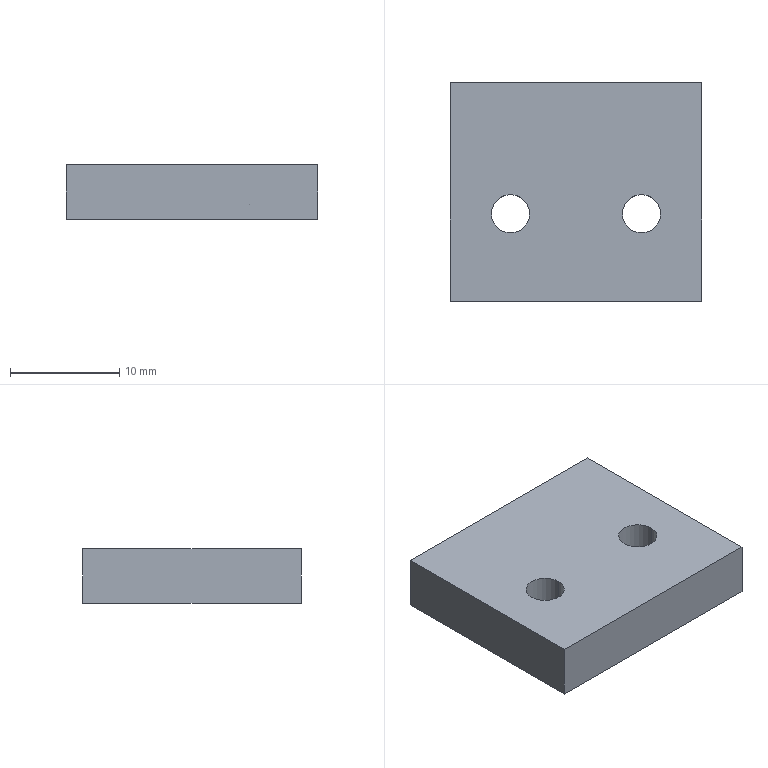Part | STEP file | Shift cylinder pad | 1 solid | 10 faces | box 23 x 20 x 5 mm | volume 2204 mm3 | plane 6 | cylinder 4 | commonest cylinder face diameters 3.5 x4
STEP:
#1=CARTESIAN_POINT('',(0.,0.,0.));
#2=DIRECTION('',(0.,0.,1.));
#3=DIRECTION('',(1.,0.,0.));
#4=AXIS2_PLACEMENT_3D('',#1,#2,#3);
#5=CARTESIAN_POINT('',(7.25,8.,0.));
#6=VERTEX_POINT('',#5);
#7=CARTESIAN_POINT('',(7.25,8.,5.));
#8=VERTEX_POINT('',#7);
#9=CARTESIAN_POINT('',(7.25,8.,0.));
#10=DIRECTION('',(0.,0.,1.));
#11=VECTOR('',#10,1.);
#12=LINE('',#9,#11);
#13=CARTESIAN_POINT('',(5.5,8.,0.));
#14=DIRECTION('',(0.,0.,1.));
#15=DIRECTION('',(1.,0.,0.));
#16=AXIS2_PLACEMENT_3D('',#13,#14,#15);
#17=CYLINDRICAL_SURFACE('',#16,1.75);
#18=CARTESIAN_POINT('',(6.283,0.));
#19=DIRECTION('',(0.,1.));
#20=VECTOR('',#19,1.);
#21=LINE('',#18,#20);
#22=(GEOMETRIC_REPRESENTATION_CONTEXT(2)PARAMETRIC_REPRESENTATION_CONTEXT()REPRESENTATION_CONTEXT('',''));
#23=DEFINITIONAL_REPRESENTATION('',(#21),#22);
#24=PCURVE('',#17,#23);
#25=CARTESIAN_POINT('',(5.5,8.,0.));
#26=DIRECTION('',(0.,0.,1.));
#27=DIRECTION('',(1.,0.,0.));
#28=AXIS2_PLACEMENT_3D('',#25,#26,#27);
#29=CYLINDRICAL_SURFACE('',#28,1.75);
#30=CARTESIAN_POINT('',(0.,0.));
#31=DIRECTION('',(0.,1.));
#32=VECTOR('',#31,1.);
#33=LINE('',#30,#32);
#34=(GEOMETRIC_REPRESENTATION_CONTEXT(2)PARAMETRIC_REPRESENTATION_CONTEXT()REPRESENTATION_CONTEXT('',''));
#35=DEFINITIONAL_REPRESENTATION('',(#33),#34);
#36=PCURVE('',#29,#35);
#37=SURFACE_CURVE('',#12,(#24,#36),.PCURVE_S1.);
#38=EDGE_CURVE('',#6,#8,#37,.T.);
#39=ORIENTED_EDGE('',*,*,#38,.T.);
#40=CARTESIAN_POINT('',(3.75,8.,5.));
#41=VERTEX_POINT('',#40);
#42=CARTESIAN_POINT('',(5.5,8.,5.));
#43=DIRECTION('',(0.,0.,1.));
#44=DIRECTION('',(1.,0.,0.));
#45=AXIS2_PLACEMENT_3D('',#42,#43,#44);
#46=CIRCLE('',#45,1.75);
#47=CARTESIAN_POINT('',(0.,5.));
#48=DIRECTION('',(1.,0.));
#49=VECTOR('',#48,1.);
#50=LINE('',#47,#49);
#51=(GEOMETRIC_REPRESENTATION_CONTEXT(2)PARAMETRIC_REPRESENTATION_CONTEXT()REPRESENTATION_CONTEXT('',''));
#52=DEFINITIONAL_REPRESENTATION('',(#50),#51);
#53=PCURVE('',#17,#52);
#54=CARTESIAN_POINT('',(0.,20.,5.));
#55=DIRECTION('',(0.,0.,-1.));
#56=DIRECTION('',(-1.,0.,0.));
#57=AXIS2_PLACEMENT_3D('',#54,#55,#56);
#58=PLANE('',#57);
#59=CARTESIAN_POINT('',(-7.25,-12.));
#60=CARTESIAN_POINT('',(-7.25,-8.969));
#61=CARTESIAN_POINT('',(-4.625,-10.484));
#62=CARTESIAN_POINT('',(-2.,-12.));
#63=CARTESIAN_POINT('',(-4.625,-13.516));
#64=CARTESIAN_POINT('',(-7.25,-15.031));
#65=CARTESIAN_POINT('',(-7.25,-12.));
#66=(BOUNDED_CURVE()B_SPLINE_CURVE(2,(#59,#60,#61,#62,#63,#64,#65),.UNSPECIFIED.,.T.,.F.)B_SPLINE_CURVE_WITH_KNOTS((1,2,2,2,2,1),(-2.094,0.,2.094,4.189,6.283,8.378),.UNSPECIFIED.)CURVE()GEOMETRIC_REPRESENTATION_ITEM()RATIONAL_B_SPLINE_CURVE((1.,0.5,1.,0.5,1.,0.5,1.))REPRESENTATION_ITEM(''));
#67=(GEOMETRIC_REPRESENTATION_CONTEXT(2)PARAMETRIC_REPRESENTATION_CONTEXT()REPRESENTATION_CONTEXT('',''));
#68=DEFINITIONAL_REPRESENTATION('',(#66),#67);
#69=PCURVE('',#58,#68);
#70=SURFACE_CURVE('',#46,(#53,#69),.PCURVE_S1.);
#71=EDGE_CURVE('',#41,#8,#70,.T.);
#72=ORIENTED_EDGE('',*,*,#71,.F.);
#73=CARTESIAN_POINT('',(3.75,8.,0.));
#74=VERTEX_POINT('',#73);
#75=CARTESIAN_POINT('',(3.75,8.,0.));
#76=DIRECTION('',(0.,0.,1.));
#77=VECTOR('',#76,1.);
#78=LINE('',#75,#77);
#79=CARTESIAN_POINT('',(3.142,0.));
#80=DIRECTION('',(0.,1.));
#81=VECTOR('',#80,1.);
#82=LINE('',#79,#81);
#83=(GEOMETRIC_REPRESENTATION_CONTEXT(2)PARAMETRIC_REPRESENTATION_CONTEXT()REPRESENTATION_CONTEXT('',''));
#84=DEFINITIONAL_REPRESENTATION('',(#82),#83);
#85=PCURVE('',#17,#84);
#86=CARTESIAN_POINT('',(3.142,0.));
#87=DIRECTION('',(0.,1.));
#88=VECTOR('',#87,1.);
#89=LINE('',#86,#88);
#90=(GEOMETRIC_REPRESENTATION_CONTEXT(2)PARAMETRIC_REPRESENTATION_CONTEXT()REPRESENTATION_CONTEXT('',''));
#91=DEFINITIONAL_REPRESENTATION('',(#89),#90);
#92=PCURVE('',#29,#91);
#93=SURFACE_CURVE('',#78,(#85,#92),.PCURVE_S1.);
#94=EDGE_CURVE('',#74,#41,#93,.T.);
#95=ORIENTED_EDGE('',*,*,#94,.F.);
#96=CARTESIAN_POINT('',(5.5,8.,0.));
#97=DIRECTION('',(0.,0.,1.));
#98=DIRECTION('',(1.,0.,0.));
#99=AXIS2_PLACEMENT_3D('',#96,#97,#98);
#100=CIRCLE('',#99,1.75);
#101=CARTESIAN_POINT('',(0.,0.));
#102=DIRECTION('',(1.,0.));
#103=VECTOR('',#102,1.);
#104=LINE('',#101,#103);
#105=(GEOMETRIC_REPRESENTATION_CONTEXT(2)PARAMETRIC_REPRESENTATION_CONTEXT()REPRESENTATION_CONTEXT('',''));
#106=DEFINITIONAL_REPRESENTATION('',(#104),#105);
#107=PCURVE('',#17,#106);
#108=CARTESIAN_POINT('',(0.,20.,0.));
#109=DIRECTION('',(0.,0.,-1.));
#110=DIRECTION('',(-1.,0.,0.));
#111=AXIS2_PLACEMENT_3D('',#108,#109,#110);
#112=PLANE('',#111);
#113=CARTESIAN_POINT('',(-7.25,-12.));
#114=CARTESIAN_POINT('',(-7.25,-8.969));
#115=CARTESIAN_POINT('',(-4.625,-10.484));
#116=CARTESIAN_POINT('',(-2.,-12.));
#117=CARTESIAN_POINT('',(-4.625,-13.516));
#118=CARTESIAN_POINT('',(-7.25,-15.031));
#119=CARTESIAN_POINT('',(-7.25,-12.));
#120=(BOUNDED_CURVE()B_SPLINE_CURVE(2,(#113,#114,#115,#116,#117,#118,#119),.UNSPECIFIED.,.T.,.F.)B_SPLINE_CURVE_WITH_KNOTS((1,2,2,2,2,1),(-2.094,0.,2.094,4.189,6.283,8.378),.UNSPECIFIED.)CURVE()GEOMETRIC_REPRESENTATION_ITEM()RATIONAL_B_SPLINE_CURVE((1.,0.5,1.,0.5,1.,0.5,1.))REPRESENTATION_ITEM(''));
#121=(GEOMETRIC_REPRESENTATION_CONTEXT(2)PARAMETRIC_REPRESENTATION_CONTEXT()REPRESENTATION_CONTEXT('',''));
#122=DEFINITIONAL_REPRESENTATION('',(#120),#121);
#123=PCURVE('',#112,#122);
#124=SURFACE_CURVE('',#100,(#107,#123),.PCURVE_S1.);
#125=EDGE_CURVE('',#74,#6,#124,.T.);
#126=ORIENTED_EDGE('',*,*,#125,.T.);
#127=EDGE_LOOP('',(#39,#72,#95,#126));
#128=FACE_BOUND('',#127,.F.);
#129=ADVANCED_FACE('',(#128),#17,.F.);
#130=CARTESIAN_POINT('',(19.25,8.,0.));
#131=VERTEX_POINT('',#130);
#132=CARTESIAN_POINT('',(19.25,8.,5.));
#133=VERTEX_POINT('',#132);
#134=CARTESIAN_POINT('',(19.25,8.,0.));
#135=DIRECTION('',(0.,0.,1.));
#136=VECTOR('',#135,1.);
#137=LINE('',#134,#136);
#138=CARTESIAN_POINT('',(17.5,8.,0.));
#139=DIRECTION('',(0.,0.,1.));
#140=DIRECTION('',(1.,0.,0.));
#141=AXIS2_PLACEMENT_3D('',#138,#139,#140);
#142=CYLINDRICAL_SURFACE('',#141,1.75);
#143=CARTESIAN_POINT('',(6.283,0.));
#144=DIRECTION('',(0.,1.));
#145=VECTOR('',#144,1.);
#146=LINE('',#143,#145);
#147=(GEOMETRIC_REPRESENTATION_CONTEXT(2)PARAMETRIC_REPRESENTATION_CONTEXT()REPRESENTATION_CONTEXT('',''));
#148=DEFINITIONAL_REPRESENTATION('',(#146),#147);
#149=PCURVE('',#142,#148);
#150=CARTESIAN_POINT('',(17.5,8.,0.));
#151=DIRECTION('',(0.,0.,1.));
#152=DIRECTION('',(1.,0.,0.));
#153=AXIS2_PLACEMENT_3D('',#150,#151,#152);
#154=CYLINDRICAL_SURFACE('',#153,1.75);
#155=CARTESIAN_POINT('',(0.,0.));
#156=DIRECTION('',(0.,1.));
#157=VECTOR('',#156,1.);
#158=LINE('',#155,#157);
#159=(GEOMETRIC_REPRESENTATION_CONTEXT(2)PARAMETRIC_REPRESENTATION_CONTEXT()REPRESENTATION_CONTEXT('',''));
#160=DEFINITIONAL_REPRESENTATION('',(#158),#159);
#161=PCURVE('',#154,#160);
#162=SURFACE_CURVE('',#137,(#149,#161),.PCURVE_S1.);
#163=EDGE_CURVE('',#131,#133,#162,.T.);
#164=ORIENTED_EDGE('',*,*,#163,.T.);
#165=CARTESIAN_POINT('',(15.75,8.,5.));
#166=VERTEX_POINT('',#165);
#167=CARTESIAN_POINT('',(17.5,8.,5.));
#168=DIRECTION('',(0.,0.,1.));
#169=DIRECTION('',(1.,0.,0.));
#170=AXIS2_PLACEMENT_3D('',#167,#168,#169);
#171=CIRCLE('',#170,1.75);
#172=CARTESIAN_POINT('',(0.,5.));
#173=DIRECTION('',(1.,0.));
#174=VECTOR('',#173,1.);
#175=LINE('',#172,#174);
#176=(GEOMETRIC_REPRESENTATION_CONTEXT(2)PARAMETRIC_REPRESENTATION_CONTEXT()REPRESENTATION_CONTEXT('',''));
#177=DEFINITIONAL_REPRESENTATION('',(#175),#176);
#178=PCURVE('',#142,#177);
#179=CARTESIAN_POINT('',(-19.25,-12.));
#180=CARTESIAN_POINT('',(-19.25,-8.969));
#181=CARTESIAN_POINT('',(-16.625,-10.484));
#182=CARTESIAN_POINT('',(-14.,-12.));
#183=CARTESIAN_POINT('',(-16.625,-13.516));
#184=CARTESIAN_POINT('',(-19.25,-15.031));
#185=CARTESIAN_POINT('',(-19.25,-12.));
#186=(BOUNDED_CURVE()B_SPLINE_CURVE(2,(#179,#180,#181,#182,#183,#184,#185),.UNSPECIFIED.,.T.,.F.)B_SPLINE_CURVE_WITH_KNOTS((1,2,2,2,2,1),(-2.094,0.,2.094,4.189,6.283,8.378),.UNSPECIFIED.)CURVE()GEOMETRIC_REPRESENTATION_ITEM()RATIONAL_B_SPLINE_CURVE((1.,0.5,1.,0.5,1.,0.5,1.))REPRESENTATION_ITEM(''));
#187=(GEOMETRIC_REPRESENTATION_CONTEXT(2)PARAMETRIC_REPRESENTATION_CONTEXT()REPRESENTATION_CONTEXT('',''));
#188=DEFINITIONAL_REPRESENTATION('',(#186),#187);
#189=PCURVE('',#58,#188);
#190=SURFACE_CURVE('',#171,(#178,#189),.PCURVE_S1.);
#191=EDGE_CURVE('',#166,#133,#190,.T.);
#192=ORIENTED_EDGE('',*,*,#191,.F.);
#193=CARTESIAN_POINT('',(15.75,8.,0.));
#194=VERTEX_POINT('',#193);
#195=CARTESIAN_POINT('',(15.75,8.,0.));
#196=DIRECTION('',(0.,0.,1.));
#197=VECTOR('',#196,1.);
#198=LINE('',#195,#197);
#199=CARTESIAN_POINT('',(3.142,0.));
#200=DIRECTION('',(0.,1.));
#201=VECTOR('',#200,1.);
#202=LINE('',#199,#201);
#203=(GEOMETRIC_REPRESENTATION_CONTEXT(2)PARAMETRIC_REPRESENTATION_CONTEXT()REPRESENTATION_CONTEXT('',''));
#204=DEFINITIONAL_REPRESENTATION('',(#202),#203);
#205=PCURVE('',#142,#204);
#206=CARTESIAN_POINT('',(3.142,0.));
#207=DIRECTION('',(0.,1.));
#208=VECTOR('',#207,1.);
#209=LINE('',#206,#208);
#210=(GEOMETRIC_REPRESENTATION_CONTEXT(2)PARAMETRIC_REPRESENTATION_CONTEXT()REPRESENTATION_CONTEXT('',''));
#211=DEFINITIONAL_REPRESENTATION('',(#209),#210);
#212=PCURVE('',#154,#211);
#213=SURFACE_CURVE('',#198,(#205,#212),.PCURVE_S1.);
#214=EDGE_CURVE('',#194,#166,#213,.T.);
#215=ORIENTED_EDGE('',*,*,#214,.F.);
#216=CARTESIAN_POINT('',(17.5,8.,0.));
#217=DIRECTION('',(0.,0.,1.));
#218=DIRECTION('',(1.,0.,0.));
#219=AXIS2_PLACEMENT_3D('',#216,#217,#218);
#220=CIRCLE('',#219,1.75);
#221=CARTESIAN_POINT('',(0.,0.));
#222=DIRECTION('',(1.,0.));
#223=VECTOR('',#222,1.);
#224=LINE('',#221,#223);
#225=(GEOMETRIC_REPRESENTATION_CONTEXT(2)PARAMETRIC_REPRESENTATION_CONTEXT()REPRESENTATION_CONTEXT('',''));
#226=DEFINITIONAL_REPRESENTATION('',(#224),#225);
#227=PCURVE('',#142,#226);
#228=CARTESIAN_POINT('',(-19.25,-12.));
#229=CARTESIAN_POINT('',(-19.25,-8.969));
#230=CARTESIAN_POINT('',(-16.625,-10.484));
#231=CARTESIAN_POINT('',(-14.,-12.));
#232=CARTESIAN_POINT('',(-16.625,-13.516));
#233=CARTESIAN_POINT('',(-19.25,-15.031));
#234=CARTESIAN_POINT('',(-19.25,-12.));
#235=(BOUNDED_CURVE()B_SPLINE_CURVE(2,(#228,#229,#230,#231,#232,#233,#234),.UNSPECIFIED.,.T.,.F.)B_SPLINE_CURVE_WITH_KNOTS((1,2,2,2,2,1),(-2.094,0.,2.094,4.189,6.283,8.378),.UNSPECIFIED.)CURVE()GEOMETRIC_REPRESENTATION_ITEM()RATIONAL_B_SPLINE_CURVE((1.,0.5,1.,0.5,1.,0.5,1.))REPRESENTATION_ITEM(''));
#236=(GEOMETRIC_REPRESENTATION_CONTEXT(2)PARAMETRIC_REPRESENTATION_CONTEXT()REPRESENTATION_CONTEXT('',''));
#237=DEFINITIONAL_REPRESENTATION('',(#235),#236);
#238=PCURVE('',#112,#237);
#239=SURFACE_CURVE('',#220,(#227,#238),.PCURVE_S1.);
#240=EDGE_CURVE('',#194,#131,#239,.T.);
#241=ORIENTED_EDGE('',*,*,#240,.T.);
#242=EDGE_LOOP('',(#164,#192,#215,#241));
#243=FACE_BOUND('',#242,.F.);
#244=ADVANCED_FACE('',(#243),#142,.F.);
#245=CARTESIAN_POINT('',(0.,20.,0.));
#246=VERTEX_POINT('',#245);
#247=CARTESIAN_POINT('',(0.,0.,0.));
#248=VERTEX_POINT('',#247);
#249=CARTESIAN_POINT('',(0.,0.,0.));
#250=DIRECTION('',(0.,-1.,0.));
#251=VECTOR('',#250,1.);
#252=LINE('',#249,#251);
#253=CARTESIAN_POINT('',(0.,0.,5.));
#254=DIRECTION('',(1.,0.,0.));
#255=DIRECTION('',(0.,0.,-1.));
#256=AXIS2_PLACEMENT_3D('',#253,#254,#255);
#257=PLANE('',#256);
#258=CARTESIAN_POINT('',(5.,0.));
#259=DIRECTION('',(0.,-1.));
#260=VECTOR('',#259,1.);
#261=LINE('',#258,#260);
#262=(GEOMETRIC_REPRESENTATION_CONTEXT(2)PARAMETRIC_REPRESENTATION_CONTEXT()REPRESENTATION_CONTEXT('',''));
#263=DEFINITIONAL_REPRESENTATION('',(#261),#262);
#264=PCURVE('',#257,#263);
#265=CARTESIAN_POINT('',(0.,-20.));
#266=DIRECTION('',(0.,-1.));
#267=VECTOR('',#266,1.);
#268=LINE('',#265,#267);
#269=(GEOMETRIC_REPRESENTATION_CONTEXT(2)PARAMETRIC_REPRESENTATION_CONTEXT()REPRESENTATION_CONTEXT('',''));
#270=DEFINITIONAL_REPRESENTATION('',(#268),#269);
#271=PCURVE('',#112,#270);
#272=SURFACE_CURVE('',#252,(#264,#271),.PCURVE_S1.);
#273=EDGE_CURVE('',#246,#248,#272,.T.);
#274=ORIENTED_EDGE('',*,*,#273,.T.);
#275=CARTESIAN_POINT('',(0.,0.,5.));
#276=VERTEX_POINT('',#275);
#277=CARTESIAN_POINT('',(0.,0.,5.));
#278=DIRECTION('',(0.,0.,-1.));
#279=VECTOR('',#278,1.);
#280=LINE('',#277,#279);
#281=CARTESIAN_POINT('',(0.,0.));
#282=DIRECTION('',(1.,0.));
#283=VECTOR('',#282,1.);
#284=LINE('',#281,#283);
#285=(GEOMETRIC_REPRESENTATION_CONTEXT(2)PARAMETRIC_REPRESENTATION_CONTEXT()REPRESENTATION_CONTEXT('',''));
#286=DEFINITIONAL_REPRESENTATION('',(#284),#285);
#287=PCURVE('',#257,#286);
#288=CARTESIAN_POINT('',(0.,0.,5.));
#289=DIRECTION('',(0.,1.,0.));
#290=DIRECTION('',(0.,0.,1.));
#291=AXIS2_PLACEMENT_3D('',#288,#289,#290);
#292=PLANE('',#291);
#293=CARTESIAN_POINT('',(0.,0.));
#294=DIRECTION('',(-1.,0.));
#295=VECTOR('',#294,1.);
#296=LINE('',#293,#295);
#297=(GEOMETRIC_REPRESENTATION_CONTEXT(2)PARAMETRIC_REPRESENTATION_CONTEXT()REPRESENTATION_CONTEXT('',''));
#298=DEFINITIONAL_REPRESENTATION('',(#296),#297);
#299=PCURVE('',#292,#298);
#300=SURFACE_CURVE('',#280,(#287,#299),.PCURVE_S1.);
#301=EDGE_CURVE('',#276,#248,#300,.T.);
#302=ORIENTED_EDGE('',*,*,#301,.F.);
#303=CARTESIAN_POINT('',(0.,20.,5.));
#304=VERTEX_POINT('',#303);
#305=CARTESIAN_POINT('',(0.,0.,5.));
#306=DIRECTION('',(0.,-1.,0.));
#307=VECTOR('',#306,1.);
#308=LINE('',#305,#307);
#309=CARTESIAN_POINT('',(0.,0.));
#310=DIRECTION('',(0.,-1.));
#311=VECTOR('',#310,1.);
#312=LINE('',#309,#311);
#313=(GEOMETRIC_REPRESENTATION_CONTEXT(2)PARAMETRIC_REPRESENTATION_CONTEXT()REPRESENTATION_CONTEXT('',''));
#314=DEFINITIONAL_REPRESENTATION('',(#312),#313);
#315=PCURVE('',#257,#314);
#316=CARTESIAN_POINT('',(0.,-20.));
#317=DIRECTION('',(0.,-1.));
#318=VECTOR('',#317,1.);
#319=LINE('',#316,#318);
#320=(GEOMETRIC_REPRESENTATION_CONTEXT(2)PARAMETRIC_REPRESENTATION_CONTEXT()REPRESENTATION_CONTEXT('',''));
#321=DEFINITIONAL_REPRESENTATION('',(#319),#320);
#322=PCURVE('',#58,#321);
#323=SURFACE_CURVE('',#308,(#315,#322),.PCURVE_S1.);
#324=EDGE_CURVE('',#304,#276,#323,.T.);
#325=ORIENTED_EDGE('',*,*,#324,.F.);
#326=CARTESIAN_POINT('',(0.,20.,5.));
#327=DIRECTION('',(0.,0.,-1.));
#328=VECTOR('',#327,1.);
#329=LINE('',#326,#328);
#330=CARTESIAN_POINT('',(0.,20.));
#331=DIRECTION('',(1.,0.));
#332=VECTOR('',#331,1.);
#333=LINE('',#330,#332);
#334=(GEOMETRIC_REPRESENTATION_CONTEXT(2)PARAMETRIC_REPRESENTATION_CONTEXT()REPRESENTATION_CONTEXT('',''));
#335=DEFINITIONAL_REPRESENTATION('',(#333),#334);
#336=PCURVE('',#257,#335);
#337=CARTESIAN_POINT('',(0.,20.,5.));
#338=DIRECTION('',(0.,-1.,0.));
#339=DIRECTION('',(0.,0.,-1.));
#340=AXIS2_PLACEMENT_3D('',#337,#338,#339);
#341=PLANE('',#340);
#342=CARTESIAN_POINT('',(0.,0.));
#343=DIRECTION('',(1.,0.));
#344=VECTOR('',#343,1.);
#345=LINE('',#342,#344);
#346=(GEOMETRIC_REPRESENTATION_CONTEXT(2)PARAMETRIC_REPRESENTATION_CONTEXT()REPRESENTATION_CONTEXT('',''));
#347=DEFINITIONAL_REPRESENTATION('',(#345),#346);
#348=PCURVE('',#341,#347);
#349=SURFACE_CURVE('',#329,(#336,#348),.PCURVE_S1.);
#350=EDGE_CURVE('',#304,#246,#349,.T.);
#351=ORIENTED_EDGE('',*,*,#350,.T.);
#352=EDGE_LOOP('',(#274,#302,#325,#351));
#353=FACE_BOUND('',#352,.T.);
#354=ADVANCED_FACE('',(#353),#257,.F.);
#355=CARTESIAN_POINT('',(23.,0.,0.));
#356=VERTEX_POINT('',#355);
#357=CARTESIAN_POINT('',(0.,0.,0.));
#358=DIRECTION('',(1.,0.,0.));
#359=VECTOR('',#358,1.);
#360=LINE('',#357,#359);
#361=CARTESIAN_POINT('',(-5.,0.));
#362=DIRECTION('',(0.,1.));
#363=VECTOR('',#362,1.);
#364=LINE('',#361,#363);
#365=(GEOMETRIC_REPRESENTATION_CONTEXT(2)PARAMETRIC_REPRESENTATION_CONTEXT()REPRESENTATION_CONTEXT('',''));
#366=DEFINITIONAL_REPRESENTATION('',(#364),#365);
#367=PCURVE('',#292,#366);
#368=CARTESIAN_POINT('',(0.,-20.));
#369=DIRECTION('',(-1.,0.));
#370=VECTOR('',#369,1.);
#371=LINE('',#368,#370);
#372=(GEOMETRIC_REPRESENTATION_CONTEXT(2)PARAMETRIC_REPRESENTATION_CONTEXT()REPRESENTATION_CONTEXT('',''));
#373=DEFINITIONAL_REPRESENTATION('',(#371),#372);
#374=PCURVE('',#112,#373);
#375=SURFACE_CURVE('',#360,(#367,#374),.PCURVE_S1.);
#376=EDGE_CURVE('',#248,#356,#375,.T.);
#377=ORIENTED_EDGE('',*,*,#376,.T.);
#378=CARTESIAN_POINT('',(23.,0.,5.));
#379=VERTEX_POINT('',#378);
#380=CARTESIAN_POINT('',(23.,0.,5.));
#381=DIRECTION('',(0.,0.,-1.));
#382=VECTOR('',#381,1.);
#383=LINE('',#380,#382);
#384=CARTESIAN_POINT('',(0.,23.));
#385=DIRECTION('',(-1.,0.));
#386=VECTOR('',#385,1.);
#387=LINE('',#384,#386);
#388=(GEOMETRIC_REPRESENTATION_CONTEXT(2)PARAMETRIC_REPRESENTATION_CONTEXT()REPRESENTATION_CONTEXT('',''));
#389=DEFINITIONAL_REPRESENTATION('',(#387),#388);
#390=PCURVE('',#292,#389);
#391=CARTESIAN_POINT('',(23.,0.,5.));
#392=DIRECTION('',(-1.,0.,0.));
#393=DIRECTION('',(0.,0.,1.));
#394=AXIS2_PLACEMENT_3D('',#391,#392,#393);
#395=PLANE('',#394);
#396=CARTESIAN_POINT('',(0.,0.));
#397=DIRECTION('',(-1.,0.));
#398=VECTOR('',#397,1.);
#399=LINE('',#396,#398);
#400=(GEOMETRIC_REPRESENTATION_CONTEXT(2)PARAMETRIC_REPRESENTATION_CONTEXT()REPRESENTATION_CONTEXT('',''));
#401=DEFINITIONAL_REPRESENTATION('',(#399),#400);
#402=PCURVE('',#395,#401);
#403=SURFACE_CURVE('',#383,(#390,#402),.PCURVE_S1.);
#404=EDGE_CURVE('',#379,#356,#403,.T.);
#405=ORIENTED_EDGE('',*,*,#404,.F.);
#406=CARTESIAN_POINT('',(0.,0.,5.));
#407=DIRECTION('',(1.,0.,0.));
#408=VECTOR('',#407,1.);
#409=LINE('',#406,#408);
#410=CARTESIAN_POINT('',(0.,0.));
#411=DIRECTION('',(0.,1.));
#412=VECTOR('',#411,1.);
#413=LINE('',#410,#412);
#414=(GEOMETRIC_REPRESENTATION_CONTEXT(2)PARAMETRIC_REPRESENTATION_CONTEXT()REPRESENTATION_CONTEXT('',''));
#415=DEFINITIONAL_REPRESENTATION('',(#413),#414);
#416=PCURVE('',#292,#415);
#417=CARTESIAN_POINT('',(0.,-20.));
#418=DIRECTION('',(-1.,0.));
#419=VECTOR('',#418,1.);
#420=LINE('',#417,#419);
#421=(GEOMETRIC_REPRESENTATION_CONTEXT(2)PARAMETRIC_REPRESENTATION_CONTEXT()REPRESENTATION_CONTEXT('',''));
#422=DEFINITIONAL_REPRESENTATION('',(#420),#421);
#423=PCURVE('',#58,#422);
#424=SURFACE_CURVE('',#409,(#416,#423),.PCURVE_S1.);
#425=EDGE_CURVE('',#276,#379,#424,.T.);
#426=ORIENTED_EDGE('',*,*,#425,.F.);
#427=ORIENTED_EDGE('',*,*,#301,.T.);
#428=EDGE_LOOP('',(#377,#405,#426,#427));
#429=FACE_BOUND('',#428,.T.);
#430=ADVANCED_FACE('',(#429),#292,.F.);
#431=CARTESIAN_POINT('',(23.,20.,0.));
#432=VERTEX_POINT('',#431);
#433=CARTESIAN_POINT('',(23.,0.,0.));
#434=DIRECTION('',(0.,1.,0.));
#435=VECTOR('',#434,1.);
#436=LINE('',#433,#435);
#437=CARTESIAN_POINT('',(-5.,0.));
#438=DIRECTION('',(0.,1.));
#439=VECTOR('',#438,1.);
#440=LINE('',#437,#439);
#441=(GEOMETRIC_REPRESENTATION_CONTEXT(2)PARAMETRIC_REPRESENTATION_CONTEXT()REPRESENTATION_CONTEXT('',''));
#442=DEFINITIONAL_REPRESENTATION('',(#440),#441);
#443=PCURVE('',#395,#442);
#444=CARTESIAN_POINT('',(-23.,-20.));
#445=DIRECTION('',(0.,1.));
#446=VECTOR('',#445,1.);
#447=LINE('',#444,#446);
#448=(GEOMETRIC_REPRESENTATION_CONTEXT(2)PARAMETRIC_REPRESENTATION_CONTEXT()REPRESENTATION_CONTEXT('',''));
#449=DEFINITIONAL_REPRESENTATION('',(#447),#448);
#450=PCURVE('',#112,#449);
#451=SURFACE_CURVE('',#436,(#443,#450),.PCURVE_S1.);
#452=EDGE_CURVE('',#356,#432,#451,.T.);
#453=ORIENTED_EDGE('',*,*,#452,.T.);
#454=CARTESIAN_POINT('',(23.,20.,5.));
#455=VERTEX_POINT('',#454);
#456=CARTESIAN_POINT('',(23.,20.,5.));
#457=DIRECTION('',(0.,0.,-1.));
#458=VECTOR('',#457,1.);
#459=LINE('',#456,#458);
#460=CARTESIAN_POINT('',(0.,20.));
#461=DIRECTION('',(-1.,0.));
#462=VECTOR('',#461,1.);
#463=LINE('',#460,#462);
#464=(GEOMETRIC_REPRESENTATION_CONTEXT(2)PARAMETRIC_REPRESENTATION_CONTEXT()REPRESENTATION_CONTEXT('',''));
#465=DEFINITIONAL_REPRESENTATION('',(#463),#464);
#466=PCURVE('',#395,#465);
#467=CARTESIAN_POINT('',(0.,23.));
#468=DIRECTION('',(1.,0.));
#469=VECTOR('',#468,1.);
#470=LINE('',#467,#469);
#471=(GEOMETRIC_REPRESENTATION_CONTEXT(2)PARAMETRIC_REPRESENTATION_CONTEXT()REPRESENTATION_CONTEXT('',''));
#472=DEFINITIONAL_REPRESENTATION('',(#470),#471);
#473=PCURVE('',#341,#472);
#474=SURFACE_CURVE('',#459,(#466,#473),.PCURVE_S1.);
#475=EDGE_CURVE('',#455,#432,#474,.T.);
#476=ORIENTED_EDGE('',*,*,#475,.F.);
#477=CARTESIAN_POINT('',(23.,0.,5.));
#478=DIRECTION('',(0.,1.,0.));
#479=VECTOR('',#478,1.);
#480=LINE('',#477,#479);
#481=CARTESIAN_POINT('',(0.,0.));
#482=DIRECTION('',(0.,1.));
#483=VECTOR('',#482,1.);
#484=LINE('',#481,#483);
#485=(GEOMETRIC_REPRESENTATION_CONTEXT(2)PARAMETRIC_REPRESENTATION_CONTEXT()REPRESENTATION_CONTEXT('',''));
#486=DEFINITIONAL_REPRESENTATION('',(#484),#485);
#487=PCURVE('',#395,#486);
#488=CARTESIAN_POINT('',(-23.,-20.));
#489=DIRECTION('',(0.,1.));
#490=VECTOR('',#489,1.);
#491=LINE('',#488,#490);
#492=(GEOMETRIC_REPRESENTATION_CONTEXT(2)PARAMETRIC_REPRESENTATION_CONTEXT()REPRESENTATION_CONTEXT('',''));
#493=DEFINITIONAL_REPRESENTATION('',(#491),#492);
#494=PCURVE('',#58,#493);
#495=SURFACE_CURVE('',#480,(#487,#494),.PCURVE_S1.);
#496=EDGE_CURVE('',#379,#455,#495,.T.);
#497=ORIENTED_EDGE('',*,*,#496,.F.);
#498=ORIENTED_EDGE('',*,*,#404,.T.);
#499=EDGE_LOOP('',(#453,#476,#497,#498));
#500=FACE_BOUND('',#499,.T.);
#501=ADVANCED_FACE('',(#500),#395,.F.);
#502=CARTESIAN_POINT('',(0.,20.,0.));
#503=DIRECTION('',(-1.,0.,0.));
#504=VECTOR('',#503,1.);
#505=LINE('',#502,#504);
#506=CARTESIAN_POINT('',(5.,0.));
#507=DIRECTION('',(0.,-1.));
#508=VECTOR('',#507,1.);
#509=LINE('',#506,#508);
#510=(GEOMETRIC_REPRESENTATION_CONTEXT(2)PARAMETRIC_REPRESENTATION_CONTEXT()REPRESENTATION_CONTEXT('',''));
#511=DEFINITIONAL_REPRESENTATION('',(#509),#510);
#512=PCURVE('',#341,#511);
#513=CARTESIAN_POINT('',(0.,0.));
#514=DIRECTION('',(1.,0.));
#515=VECTOR('',#514,1.);
#516=LINE('',#513,#515);
#517=(GEOMETRIC_REPRESENTATION_CONTEXT(2)PARAMETRIC_REPRESENTATION_CONTEXT()REPRESENTATION_CONTEXT('',''));
#518=DEFINITIONAL_REPRESENTATION('',(#516),#517);
#519=PCURVE('',#112,#518);
#520=SURFACE_CURVE('',#505,(#512,#519),.PCURVE_S1.);
#521=EDGE_CURVE('',#432,#246,#520,.T.);
#522=ORIENTED_EDGE('',*,*,#521,.T.);
#523=ORIENTED_EDGE('',*,*,#350,.F.);
#524=CARTESIAN_POINT('',(0.,20.,5.));
#525=DIRECTION('',(-1.,0.,0.));
#526=VECTOR('',#525,1.);
#527=LINE('',#524,#526);
#528=CARTESIAN_POINT('',(0.,0.));
#529=DIRECTION('',(0.,-1.));
#530=VECTOR('',#529,1.);
#531=LINE('',#528,#530);
#532=(GEOMETRIC_REPRESENTATION_CONTEXT(2)PARAMETRIC_REPRESENTATION_CONTEXT()REPRESENTATION_CONTEXT('',''));
#533=DEFINITIONAL_REPRESENTATION('',(#531),#532);
#534=PCURVE('',#341,#533);
#535=CARTESIAN_POINT('',(0.,0.));
#536=DIRECTION('',(1.,0.));
#537=VECTOR('',#536,1.);
#538=LINE('',#535,#537);
#539=(GEOMETRIC_REPRESENTATION_CONTEXT(2)PARAMETRIC_REPRESENTATION_CONTEXT()REPRESENTATION_CONTEXT('',''));
#540=DEFINITIONAL_REPRESENTATION('',(#538),#539);
#541=PCURVE('',#58,#540);
#542=SURFACE_CURVE('',#527,(#534,#541),.PCURVE_S1.);
#543=EDGE_CURVE('',#455,#304,#542,.T.);
#544=ORIENTED_EDGE('',*,*,#543,.F.);
#545=ORIENTED_EDGE('',*,*,#475,.T.);
#546=EDGE_LOOP('',(#522,#523,#544,#545));
#547=FACE_BOUND('',#546,.T.);
#548=ADVANCED_FACE('',(#547),#341,.F.);
#549=CARTESIAN_POINT('',(5.5,8.,5.));
#550=DIRECTION('',(0.,0.,1.));
#551=DIRECTION('',(1.,0.,0.));
#552=AXIS2_PLACEMENT_3D('',#549,#550,#551);
#553=CIRCLE('',#552,1.75);
#554=CARTESIAN_POINT('',(-7.25,-12.));
#555=CARTESIAN_POINT('',(-7.25,-8.969));
#556=CARTESIAN_POINT('',(-4.625,-10.484));
#557=CARTESIAN_POINT('',(-2.,-12.));
#558=CARTESIAN_POINT('',(-4.625,-13.516));
#559=CARTESIAN_POINT('',(-7.25,-15.031));
#560=CARTESIAN_POINT('',(-7.25,-12.));
#561=(BOUNDED_CURVE()B_SPLINE_CURVE(2,(#554,#555,#556,#557,#558,#559,#560),.UNSPECIFIED.,.T.,.F.)B_SPLINE_CURVE_WITH_KNOTS((1,2,2,2,2,1),(-2.094,0.,2.094,4.189,6.283,8.378),.UNSPECIFIED.)CURVE()GEOMETRIC_REPRESENTATION_ITEM()RATIONAL_B_SPLINE_CURVE((1.,0.5,1.,0.5,1.,0.5,1.))REPRESENTATION_ITEM(''));
#562=(GEOMETRIC_REPRESENTATION_CONTEXT(2)PARAMETRIC_REPRESENTATION_CONTEXT()REPRESENTATION_CONTEXT('',''));
#563=DEFINITIONAL_REPRESENTATION('',(#561),#562);
#564=PCURVE('',#58,#563);
#565=CARTESIAN_POINT('',(0.,5.));
#566=DIRECTION('',(1.,0.));
#567=VECTOR('',#566,1.);
#568=LINE('',#565,#567);
#569=(GEOMETRIC_REPRESENTATION_CONTEXT(2)PARAMETRIC_REPRESENTATION_CONTEXT()REPRESENTATION_CONTEXT('',''));
#570=DEFINITIONAL_REPRESENTATION('',(#568),#569);
#571=PCURVE('',#29,#570);
#572=SURFACE_CURVE('',#553,(#564,#571),.PCURVE_S1.);
#573=EDGE_CURVE('',#8,#41,#572,.T.);
#574=ORIENTED_EDGE('',*,*,#573,.F.);
#575=ORIENTED_EDGE('',*,*,#71,.F.);
#576=EDGE_LOOP('',(#574,#575));
#577=FACE_BOUND('',#576,.T.);
#578=CARTESIAN_POINT('',(17.5,8.,5.));
#579=DIRECTION('',(0.,0.,1.));
#580=DIRECTION('',(1.,0.,0.));
#581=AXIS2_PLACEMENT_3D('',#578,#579,#580);
#582=CIRCLE('',#581,1.75);
#583=CARTESIAN_POINT('',(-19.25,-12.));
#584=CARTESIAN_POINT('',(-19.25,-8.969));
#585=CARTESIAN_POINT('',(-16.625,-10.484));
#586=CARTESIAN_POINT('',(-14.,-12.));
#587=CARTESIAN_POINT('',(-16.625,-13.516));
#588=CARTESIAN_POINT('',(-19.25,-15.031));
#589=CARTESIAN_POINT('',(-19.25,-12.));
#590=(BOUNDED_CURVE()B_SPLINE_CURVE(2,(#583,#584,#585,#586,#587,#588,#589),.UNSPECIFIED.,.T.,.F.)B_SPLINE_CURVE_WITH_KNOTS((1,2,2,2,2,1),(-2.094,0.,2.094,4.189,6.283,8.378),.UNSPECIFIED.)CURVE()GEOMETRIC_REPRESENTATION_ITEM()RATIONAL_B_SPLINE_CURVE((1.,0.5,1.,0.5,1.,0.5,1.))REPRESENTATION_ITEM(''));
#591=(GEOMETRIC_REPRESENTATION_CONTEXT(2)PARAMETRIC_REPRESENTATION_CONTEXT()REPRESENTATION_CONTEXT('',''));
#592=DEFINITIONAL_REPRESENTATION('',(#590),#591);
#593=PCURVE('',#58,#592);
#594=CARTESIAN_POINT('',(0.,5.));
#595=DIRECTION('',(1.,0.));
#596=VECTOR('',#595,1.);
#597=LINE('',#594,#596);
#598=(GEOMETRIC_REPRESENTATION_CONTEXT(2)PARAMETRIC_REPRESENTATION_CONTEXT()REPRESENTATION_CONTEXT('',''));
#599=DEFINITIONAL_REPRESENTATION('',(#597),#598);
#600=PCURVE('',#154,#599);
#601=SURFACE_CURVE('',#582,(#593,#600),.PCURVE_S1.);
#602=EDGE_CURVE('',#133,#166,#601,.T.);
#603=ORIENTED_EDGE('',*,*,#602,.F.);
#604=ORIENTED_EDGE('',*,*,#191,.F.);
#605=EDGE_LOOP('',(#603,#604));
#606=FACE_BOUND('',#605,.T.);
#607=ORIENTED_EDGE('',*,*,#324,.T.);
#608=ORIENTED_EDGE('',*,*,#425,.T.);
#609=ORIENTED_EDGE('',*,*,#496,.T.);
#610=ORIENTED_EDGE('',*,*,#543,.T.);
#611=EDGE_LOOP('',(#607,#608,#609,#610));
#612=FACE_BOUND('',#611,.T.);
#613=ADVANCED_FACE('',(#577,#606,#612),#58,.F.);
#614=CARTESIAN_POINT('',(5.5,8.,0.));
#615=DIRECTION('',(0.,0.,1.));
#616=DIRECTION('',(1.,0.,0.));
#617=AXIS2_PLACEMENT_3D('',#614,#615,#616);
#618=CIRCLE('',#617,1.75);
#619=CARTESIAN_POINT('',(-7.25,-12.));
#620=CARTESIAN_POINT('',(-7.25,-8.969));
#621=CARTESIAN_POINT('',(-4.625,-10.484));
#622=CARTESIAN_POINT('',(-2.,-12.));
#623=CARTESIAN_POINT('',(-4.625,-13.516));
#624=CARTESIAN_POINT('',(-7.25,-15.031));
#625=CARTESIAN_POINT('',(-7.25,-12.));
#626=(BOUNDED_CURVE()B_SPLINE_CURVE(2,(#619,#620,#621,#622,#623,#624,#625),.UNSPECIFIED.,.T.,.F.)B_SPLINE_CURVE_WITH_KNOTS((1,2,2,2,2,1),(-2.094,0.,2.094,4.189,6.283,8.378),.UNSPECIFIED.)CURVE()GEOMETRIC_REPRESENTATION_ITEM()RATIONAL_B_SPLINE_CURVE((1.,0.5,1.,0.5,1.,0.5,1.))REPRESENTATION_ITEM(''));
#627=(GEOMETRIC_REPRESENTATION_CONTEXT(2)PARAMETRIC_REPRESENTATION_CONTEXT()REPRESENTATION_CONTEXT('',''));
#628=DEFINITIONAL_REPRESENTATION('',(#626),#627);
#629=PCURVE('',#112,#628);
#630=CARTESIAN_POINT('',(0.,0.));
#631=DIRECTION('',(1.,0.));
#632=VECTOR('',#631,1.);
#633=LINE('',#630,#632);
#634=(GEOMETRIC_REPRESENTATION_CONTEXT(2)PARAMETRIC_REPRESENTATION_CONTEXT()REPRESENTATION_CONTEXT('',''));
#635=DEFINITIONAL_REPRESENTATION('',(#633),#634);
#636=PCURVE('',#29,#635);
#637=SURFACE_CURVE('',#618,(#629,#636),.PCURVE_S1.);
#638=EDGE_CURVE('',#6,#74,#637,.T.);
#639=ORIENTED_EDGE('',*,*,#638,.T.);
#640=ORIENTED_EDGE('',*,*,#125,.T.);
#641=EDGE_LOOP('',(#639,#640));
#642=FACE_BOUND('',#641,.T.);
#643=CARTESIAN_POINT('',(17.5,8.,0.));
#644=DIRECTION('',(0.,0.,1.));
#645=DIRECTION('',(1.,0.,0.));
#646=AXIS2_PLACEMENT_3D('',#643,#644,#645);
#647=CIRCLE('',#646,1.75);
#648=CARTESIAN_POINT('',(-19.25,-12.));
#649=CARTESIAN_POINT('',(-19.25,-8.969));
#650=CARTESIAN_POINT('',(-16.625,-10.484));
#651=CARTESIAN_POINT('',(-14.,-12.));
#652=CARTESIAN_POINT('',(-16.625,-13.516));
#653=CARTESIAN_POINT('',(-19.25,-15.031));
#654=CARTESIAN_POINT('',(-19.25,-12.));
#655=(BOUNDED_CURVE()B_SPLINE_CURVE(2,(#648,#649,#650,#651,#652,#653,#654),.UNSPECIFIED.,.T.,.F.)B_SPLINE_CURVE_WITH_KNOTS((1,2,2,2,2,1),(-2.094,0.,2.094,4.189,6.283,8.378),.UNSPECIFIED.)CURVE()GEOMETRIC_REPRESENTATION_ITEM()RATIONAL_B_SPLINE_CURVE((1.,0.5,1.,0.5,1.,0.5,1.))REPRESENTATION_ITEM(''));
#656=(GEOMETRIC_REPRESENTATION_CONTEXT(2)PARAMETRIC_REPRESENTATION_CONTEXT()REPRESENTATION_CONTEXT('',''));
#657=DEFINITIONAL_REPRESENTATION('',(#655),#656);
#658=PCURVE('',#112,#657);
#659=CARTESIAN_POINT('',(0.,0.));
#660=DIRECTION('',(1.,0.));
#661=VECTOR('',#660,1.);
#662=LINE('',#659,#661);
#663=(GEOMETRIC_REPRESENTATION_CONTEXT(2)PARAMETRIC_REPRESENTATION_CONTEXT()REPRESENTATION_CONTEXT('',''));
#664=DEFINITIONAL_REPRESENTATION('',(#662),#663);
#665=PCURVE('',#154,#664);
#666=SURFACE_CURVE('',#647,(#658,#665),.PCURVE_S1.);
#667=EDGE_CURVE('',#131,#194,#666,.T.);
#668=ORIENTED_EDGE('',*,*,#667,.T.);
#669=ORIENTED_EDGE('',*,*,#240,.T.);
#670=EDGE_LOOP('',(#668,#669));
#671=FACE_BOUND('',#670,.T.);
#672=ORIENTED_EDGE('',*,*,#273,.F.);
#673=ORIENTED_EDGE('',*,*,#521,.F.);
#674=ORIENTED_EDGE('',*,*,#452,.F.);
#675=ORIENTED_EDGE('',*,*,#376,.F.);
#676=EDGE_LOOP('',(#672,#673,#674,#675));
#677=FACE_BOUND('',#676,.T.);
#678=ADVANCED_FACE('',(#642,#671,#677),#112,.T.);
#679=ORIENTED_EDGE('',*,*,#602,.F.);
#680=ORIENTED_EDGE('',*,*,#163,.F.);
#681=ORIENTED_EDGE('',*,*,#667,.T.);
#682=ORIENTED_EDGE('',*,*,#214,.T.);
#683=EDGE_LOOP('',(#679,#680,#681,#682));
#684=FACE_BOUND('',#683,.F.);
#685=ADVANCED_FACE('',(#684),#154,.F.);
#686=ORIENTED_EDGE('',*,*,#573,.F.);
#687=ORIENTED_EDGE('',*,*,#38,.F.);
#688=ORIENTED_EDGE('',*,*,#638,.T.);
#689=ORIENTED_EDGE('',*,*,#94,.T.);
#690=EDGE_LOOP('',(#686,#687,#688,#689));
#691=FACE_BOUND('',#690,.F.);
#692=ADVANCED_FACE('',(#691),#29,.F.);
#693=CLOSED_SHELL('',(#129,#244,#354,#430,#501,#548,#613,#678,#685,#692));
#694=MANIFOLD_SOLID_BREP('',#693);
#695=(LENGTH_UNIT()NAMED_UNIT(*)SI_UNIT(.MILLI.,.METRE.));
#696=UNCERTAINTY_MEASURE_WITH_UNIT(LENGTH_MEASURE(0.0000001),#695,'','');
#697=(NAMED_UNIT(*)PLANE_ANGLE_UNIT()SI_UNIT($,.RADIAN.));
#698=(NAMED_UNIT(*)SI_UNIT($,.STERADIAN.)SOLID_ANGLE_UNIT());
#699=(GEOMETRIC_REPRESENTATION_CONTEXT(3)GLOBAL_UNCERTAINTY_ASSIGNED_CONTEXT((#696))GLOBAL_UNIT_ASSIGNED_CONTEXT((#695,#697,#698))REPRESENTATION_CONTEXT('',''));
#700=ADVANCED_BREP_SHAPE_REPRESENTATION('',(#4,#694),#699);